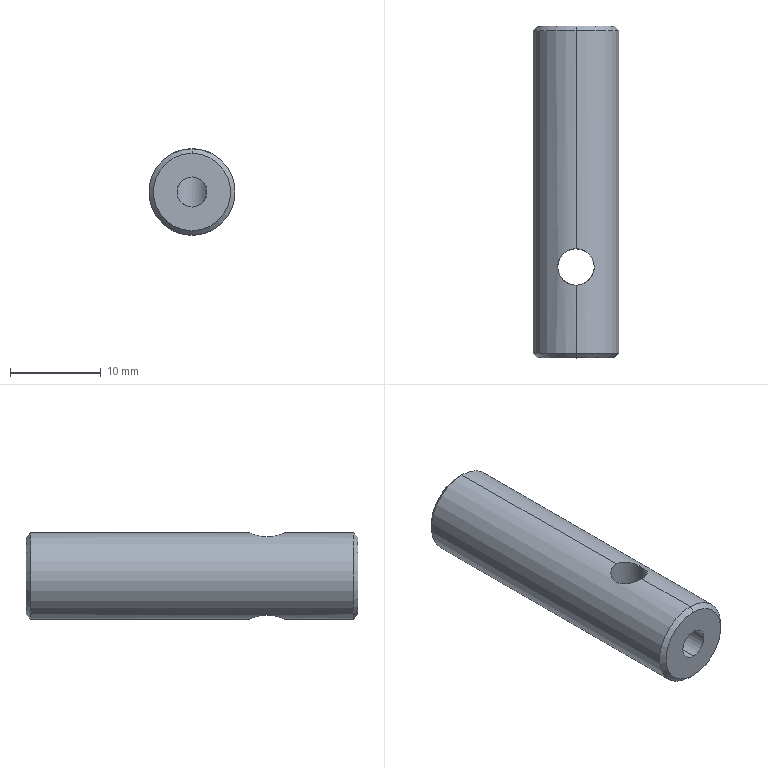Part | STEP file | PN_0050 | 1 solid | 16 faces | box 9.5 x 36.5 x 9.5 mm | volume 2304 mm3 | cylinder 8 | cone 6 | plane 2 | commonest cylinder face diameters 3.3 x4 4 x2 9.5 x2